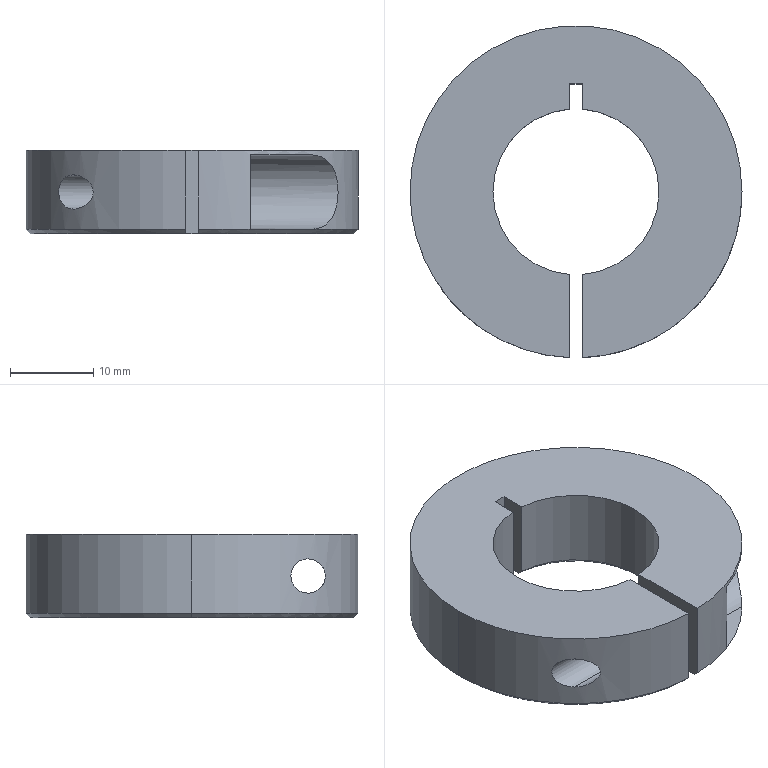Part | STEP file | qnSceond1_10 | 1 solid | 27 faces | box 40 x 39.986 x 10 mm | volume 8415 mm3 | cylinder 11 | plane 10 | cone 6 | commonest cylinder face diameters 20 x3 40 x3 4.134 x2 5.5 x2 9 x1